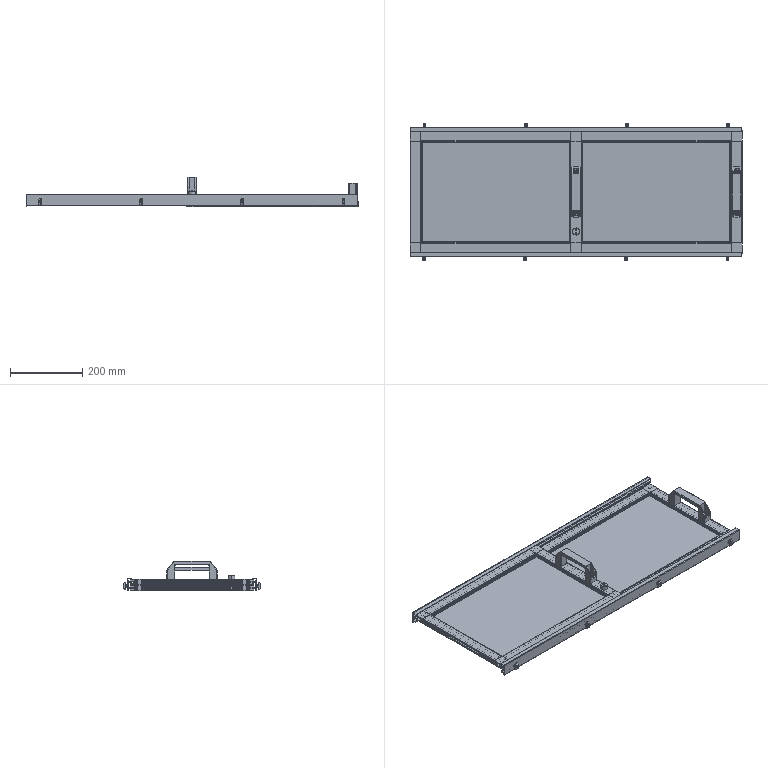Part | NX | features BREP 18 | 69 solids | 2339 faces | box 920 x 379 x 81 mm | volume 2027071 mm3 | plane 1438 | cylinder 629 | cone 172 | torus 84 | spline 8 | sphere 8 | commonest cylinder face diameters 5 x90 1 x84 2 x64 11 x64 0.4 x48 8 x46